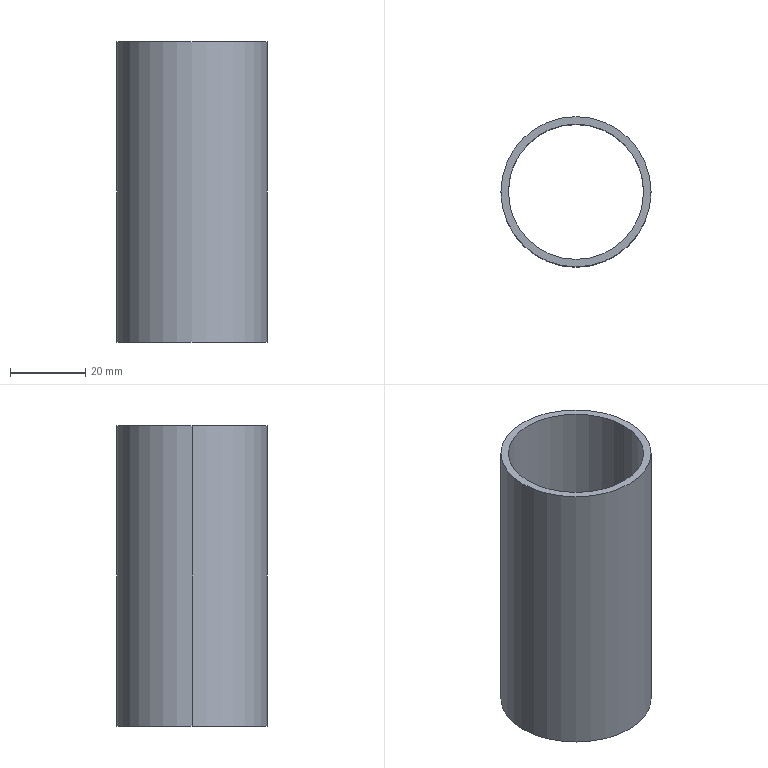Part | SolidWorks | features Extrusion 1 | 1 solid | 6 faces | box 40 x 40 x 80 mm | volume 19101 mm3 | cylinder 4 | plane 2 | commonest cylinder face diameters 36 x2 40 x2
STEP:
#1=CARTESIAN_POINT('',(-18.,0.,-40.));
#2=VERTEX_POINT('',#1);
#3=CARTESIAN_POINT('',(18.,0.,-40.));
#4=VERTEX_POINT('',#3);
#5=CARTESIAN_POINT('',(0.,0.,-40.));
#6=DIRECTION('',(0.,0.,1.));
#7=DIRECTION('',(1.,0.,0.));
#8=AXIS2_PLACEMENT_3D('',#5,#6,#7);
#9=CIRCLE('',#8,18.);
#10=EDGE_CURVE('',#2,#4,#9,.T.);
#11=ORIENTED_EDGE('',*,*,#10,.F.);
#12=CARTESIAN_POINT('',(-18.,0.,40.));
#13=VERTEX_POINT('',#12);
#14=CARTESIAN_POINT('',(-18.,0.,-40.));
#15=DIRECTION('',(0.,0.,1.));
#16=VECTOR('',#15,1000.);
#17=LINE('',#14,#16);
#18=EDGE_CURVE('',#2,#13,#17,.T.);
#19=ORIENTED_EDGE('',*,*,#18,.T.);
#20=CARTESIAN_POINT('',(18.,0.,40.));
#21=VERTEX_POINT('',#20);
#22=CARTESIAN_POINT('',(0.,0.,40.));
#23=DIRECTION('',(0.,0.,1.));
#24=DIRECTION('',(1.,0.,0.));
#25=AXIS2_PLACEMENT_3D('',#22,#23,#24);
#26=CIRCLE('',#25,18.);
#27=EDGE_CURVE('',#13,#21,#26,.T.);
#28=ORIENTED_EDGE('',*,*,#27,.T.);
#29=CARTESIAN_POINT('',(18.,0.,-40.));
#30=DIRECTION('',(0.,0.,1.));
#31=VECTOR('',#30,1000.);
#32=LINE('',#29,#31);
#33=EDGE_CURVE('',#4,#21,#32,.T.);
#34=ORIENTED_EDGE('',*,*,#33,.F.);
#35=EDGE_LOOP('',(#11,#19,#28,#34));
#36=FACE_OUTER_BOUND('',#35,.T.);
#37=CARTESIAN_POINT('',(0.,0.,-40.));
#38=DIRECTION('',(0.,0.,1.));
#39=DIRECTION('',(1.,0.,0.));
#40=AXIS2_PLACEMENT_3D('',#37,#38,#39);
#41=CYLINDRICAL_SURFACE('',#40,18.);
#42=ADVANCED_FACE('',(#36),#41,.F.);
#43=CARTESIAN_POINT('',(20.,0.,-40.));
#44=VERTEX_POINT('',#43);
#45=CARTESIAN_POINT('',(-20.,0.,-40.));
#46=VERTEX_POINT('',#45);
#47=CARTESIAN_POINT('',(0.,0.,-40.));
#48=DIRECTION('',(0.,0.,1.));
#49=DIRECTION('',(1.,0.,0.));
#50=AXIS2_PLACEMENT_3D('',#47,#48,#49);
#51=CIRCLE('',#50,20.);
#52=EDGE_CURVE('',#44,#46,#51,.T.);
#53=ORIENTED_EDGE('',*,*,#52,.T.);
#54=CARTESIAN_POINT('',(-20.,0.,40.));
#55=VERTEX_POINT('',#54);
#56=CARTESIAN_POINT('',(-20.,0.,-40.));
#57=DIRECTION('',(0.,0.,1.));
#58=VECTOR('',#57,1000.);
#59=LINE('',#56,#58);
#60=EDGE_CURVE('',#46,#55,#59,.T.);
#61=ORIENTED_EDGE('',*,*,#60,.T.);
#62=CARTESIAN_POINT('',(20.,0.,40.));
#63=VERTEX_POINT('',#62);
#64=CARTESIAN_POINT('',(0.,0.,40.));
#65=DIRECTION('',(0.,0.,1.));
#66=DIRECTION('',(1.,0.,0.));
#67=AXIS2_PLACEMENT_3D('',#64,#65,#66);
#68=CIRCLE('',#67,20.);
#69=EDGE_CURVE('',#63,#55,#68,.T.);
#70=ORIENTED_EDGE('',*,*,#69,.F.);
#71=CARTESIAN_POINT('',(20.,0.,-40.));
#72=DIRECTION('',(0.,0.,1.));
#73=VECTOR('',#72,1000.);
#74=LINE('',#71,#73);
#75=EDGE_CURVE('',#44,#63,#74,.T.);
#76=ORIENTED_EDGE('',*,*,#75,.F.);
#77=EDGE_LOOP('',(#53,#61,#70,#76));
#78=FACE_OUTER_BOUND('',#77,.T.);
#79=CARTESIAN_POINT('',(0.,0.,-40.));
#80=DIRECTION('',(0.,0.,1.));
#81=DIRECTION('',(1.,0.,0.));
#82=AXIS2_PLACEMENT_3D('',#79,#80,#81);
#83=CYLINDRICAL_SURFACE('',#82,20.);
#84=ADVANCED_FACE('',(#78),#83,.T.);
#85=ORIENTED_EDGE('',*,*,#60,.F.);
#86=CARTESIAN_POINT('',(0.,0.,-40.));
#87=DIRECTION('',(0.,0.,1.));
#88=DIRECTION('',(1.,0.,0.));
#89=AXIS2_PLACEMENT_3D('',#86,#87,#88);
#90=CIRCLE('',#89,20.);
#91=EDGE_CURVE('',#46,#44,#90,.T.);
#92=ORIENTED_EDGE('',*,*,#91,.T.);
#93=ORIENTED_EDGE('',*,*,#75,.T.);
#94=CARTESIAN_POINT('',(0.,0.,40.));
#95=DIRECTION('',(0.,0.,1.));
#96=DIRECTION('',(1.,0.,0.));
#97=AXIS2_PLACEMENT_3D('',#94,#95,#96);
#98=CIRCLE('',#97,20.);
#99=EDGE_CURVE('',#55,#63,#98,.T.);
#100=ORIENTED_EDGE('',*,*,#99,.F.);
#101=EDGE_LOOP('',(#85,#92,#93,#100));
#102=FACE_OUTER_BOUND('',#101,.T.);
#103=CARTESIAN_POINT('',(0.,0.,-40.));
#104=DIRECTION('',(0.,0.,1.));
#105=DIRECTION('',(1.,0.,0.));
#106=AXIS2_PLACEMENT_3D('',#103,#104,#105);
#107=CYLINDRICAL_SURFACE('',#106,20.);
#108=ADVANCED_FACE('',(#102),#107,.T.);
#109=CARTESIAN_POINT('',(0.,0.,-40.));
#110=DIRECTION('',(0.,0.,1.));
#111=DIRECTION('',(1.,0.,0.));
#112=AXIS2_PLACEMENT_3D('',#109,#110,#111);
#113=CIRCLE('',#112,18.);
#114=EDGE_CURVE('',#4,#2,#113,.T.);
#115=ORIENTED_EDGE('',*,*,#114,.T.);
#116=ORIENTED_EDGE('',*,*,#10,.T.);
#117=EDGE_LOOP('',(#115,#116));
#118=FACE_BOUND('',#117,.T.);
#119=ORIENTED_EDGE('',*,*,#52,.F.);
#120=ORIENTED_EDGE('',*,*,#91,.F.);
#121=EDGE_LOOP('',(#119,#120));
#122=FACE_OUTER_BOUND('',#121,.T.);
#123=CARTESIAN_POINT('',(0.,0.,-40.));
#124=DIRECTION('',(0.,0.,1.));
#125=DIRECTION('',(1.,0.,0.));
#126=AXIS2_PLACEMENT_3D('',#123,#124,#125);
#127=PLANE('',#126);
#128=ADVANCED_FACE('',(#118,#122),#127,.F.);
#129=CARTESIAN_POINT('',(0.,0.,40.));
#130=DIRECTION('',(0.,0.,1.));
#131=DIRECTION('',(1.,0.,0.));
#132=AXIS2_PLACEMENT_3D('',#129,#130,#131);
#133=CIRCLE('',#132,18.);
#134=EDGE_CURVE('',#21,#13,#133,.T.);
#135=ORIENTED_EDGE('',*,*,#134,.F.);
#136=ORIENTED_EDGE('',*,*,#27,.F.);
#137=EDGE_LOOP('',(#135,#136));
#138=FACE_BOUND('',#137,.T.);
#139=ORIENTED_EDGE('',*,*,#69,.T.);
#140=ORIENTED_EDGE('',*,*,#99,.T.);
#141=EDGE_LOOP('',(#139,#140));
#142=FACE_OUTER_BOUND('',#141,.T.);
#143=CARTESIAN_POINT('',(0.,0.,40.));
#144=DIRECTION('',(0.,0.,1.));
#145=DIRECTION('',(1.,0.,0.));
#146=AXIS2_PLACEMENT_3D('',#143,#144,#145);
#147=PLANE('',#146);
#148=ADVANCED_FACE('',(#138,#142),#147,.T.);
#149=ORIENTED_EDGE('',*,*,#18,.F.);
#150=ORIENTED_EDGE('',*,*,#114,.F.);
#151=ORIENTED_EDGE('',*,*,#33,.T.);
#152=ORIENTED_EDGE('',*,*,#134,.T.);
#153=EDGE_LOOP('',(#149,#150,#151,#152));
#154=FACE_OUTER_BOUND('',#153,.T.);
#155=CARTESIAN_POINT('',(0.,0.,-40.));
#156=DIRECTION('',(0.,0.,1.));
#157=DIRECTION('',(1.,0.,0.));
#158=AXIS2_PLACEMENT_3D('',#155,#156,#157);
#159=CYLINDRICAL_SURFACE('',#158,18.);
#160=ADVANCED_FACE('',(#154),#159,.F.);
#161=CLOSED_SHELL('',(#42,#84,#108,#128,#148,#160));
#162=MANIFOLD_SOLID_BREP('',#161);
#163=CARTESIAN_POINT('',(0.,0.,0.));
#164=DIRECTION('',(0.,0.,1.));
#165=DIRECTION('',(1.,0.,0.));
#166=AXIS2_PLACEMENT_3D('',#163,#164,#165);
#167=(LENGTH_UNIT()NAMED_UNIT(*)SI_UNIT(.MILLI.,.METRE.));
#168=UNCERTAINTY_MEASURE_WITH_UNIT(LENGTH_MEASURE(0.00001),#167,'','');
#169=(NAMED_UNIT(*)PLANE_ANGLE_UNIT()SI_UNIT($,.RADIAN.));
#170=(NAMED_UNIT(*)SI_UNIT($,.STERADIAN.)SOLID_ANGLE_UNIT());
#171=(GEOMETRIC_REPRESENTATION_CONTEXT(3)GLOBAL_UNCERTAINTY_ASSIGNED_CONTEXT((#168))GLOBAL_UNIT_ASSIGNED_CONTEXT((#167,#169,#170))REPRESENTATION_CONTEXT('',''));
#172=ADVANCED_BREP_SHAPE_REPRESENTATION('',(#162,#166),#171);